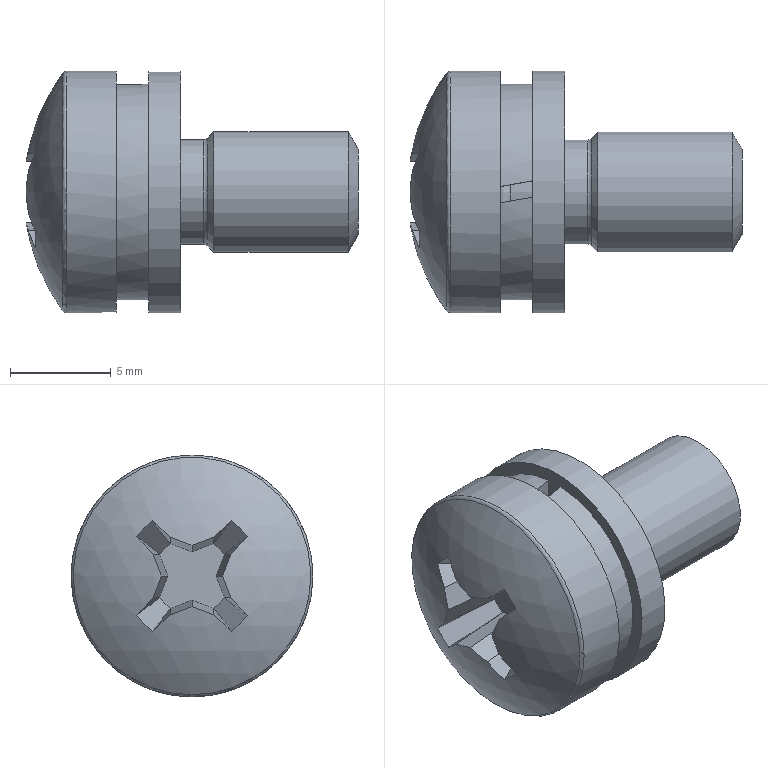Part | STEP file | Cross recessed pan head combination screw M6×12 A2-70 GBT9074.4-1988 | 3 solids | 42 faces | box 16.483 x 12 x 12 mm | volume 913.256 mm3 | plane 29 | cylinder 7 | torus 3 | cone 2 | sphere 1 | commonest cylinder face diameters 5.71 x2 12 x2 5.196 x1 6 x1 10.71 x1